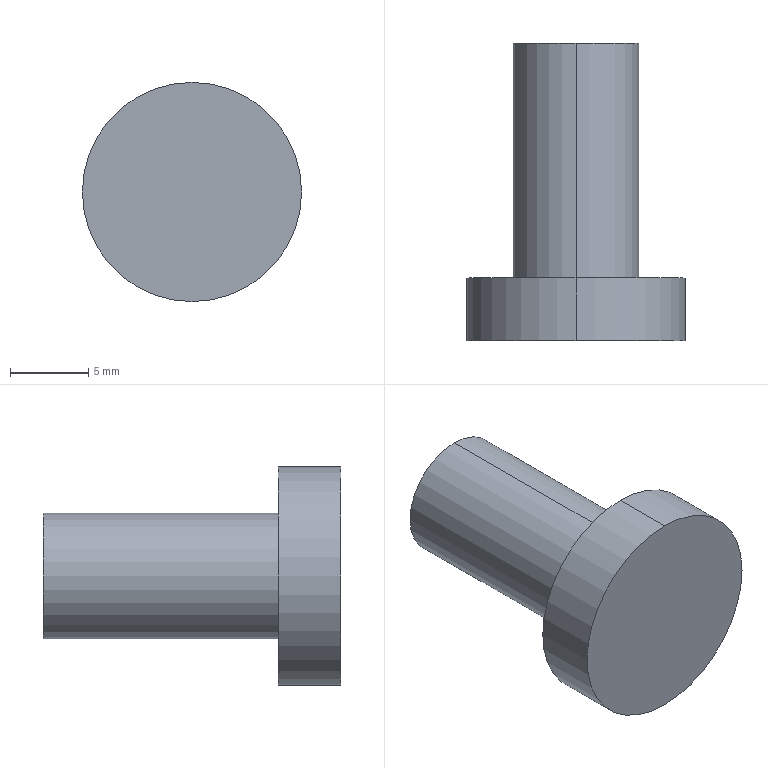Part | STEP file | BU-C03b | 1 solid | 7 faces | box 14 x 19 x 14 mm | volume 1370 mm3 | cylinder 4 | plane 3 | commonest cylinder face diameters 8 x2 14 x2
STEP:
#1=CARTESIAN_POINT('',(0.,0.,0.));
#2=DIRECTION('',(0.,0.,1.));
#3=DIRECTION('',(1.,0.,0.));
#4=AXIS2_PLACEMENT_3D('',#1,#2,#3);
#5=CARTESIAN_POINT('',(0.,4.,4.));
#6=VERTEX_POINT('',#5);
#7=CARTESIAN_POINT('',(0.,4.,-4.));
#8=VERTEX_POINT('',#7);
#9=CARTESIAN_POINT('',(0.,4.,0.));
#10=DIRECTION('',(0.,1.,0.));
#11=DIRECTION('',(0.,0.,1.));
#12=AXIS2_PLACEMENT_3D('',#9,#10,#11);
#13=CIRCLE('',#12,4.);
#14=CARTESIAN_POINT('',(0.,28.998,0.));
#15=DIRECTION('',(0.,1.,0.));
#16=DIRECTION('',(0.,0.,1.));
#17=AXIS2_PLACEMENT_3D('',#14,#15,#16);
#18=CYLINDRICAL_SURFACE('',#17,4.);
#19=CARTESIAN_POINT('',(0.,-24.998));
#20=DIRECTION('',(1.,0.));
#21=VECTOR('',#20,1.);
#22=LINE('',#19,#21);
#23=(GEOMETRIC_REPRESENTATION_CONTEXT(2)PARAMETRIC_REPRESENTATION_CONTEXT()REPRESENTATION_CONTEXT('',''));
#24=DEFINITIONAL_REPRESENTATION('',(#22),#23);
#25=PCURVE('',#18,#24);
#26=CARTESIAN_POINT('',(-4.,4.,0.));
#27=DIRECTION('',(0.,1.,0.));
#28=DIRECTION('',(0.,0.,1.));
#29=AXIS2_PLACEMENT_3D('',#26,#27,#28);
#30=PLANE('',#29);
#31=CARTESIAN_POINT('',(0.,4.));
#32=DIRECTION('',(1.,0.));
#33=AXIS2_PLACEMENT_2D('',#31,#32);
#34=CIRCLE('',#33,4.);
#35=(GEOMETRIC_REPRESENTATION_CONTEXT(2)PARAMETRIC_REPRESENTATION_CONTEXT()REPRESENTATION_CONTEXT('',''));
#36=DEFINITIONAL_REPRESENTATION('',(#34),#35);
#37=PCURVE('',#30,#36);
#38=SURFACE_CURVE('',#13,(#25,#37),.PCURVE_S1.);
#39=EDGE_CURVE('',#6,#8,#38,.T.);
#40=ORIENTED_EDGE('',*,*,#39,.T.);
#41=CARTESIAN_POINT('',(0.,19.,-4.));
#42=VERTEX_POINT('',#41);
#43=CARTESIAN_POINT('',(0.,28.998,-4.));
#44=DIRECTION('',(0.,1.,0.));
#45=VECTOR('',#44,1.);
#46=LINE('',#43,#45);
#47=CARTESIAN_POINT('',(3.142,0.));
#48=DIRECTION('',(0.,1.));
#49=VECTOR('',#48,1.);
#50=LINE('',#47,#49);
#51=(GEOMETRIC_REPRESENTATION_CONTEXT(2)PARAMETRIC_REPRESENTATION_CONTEXT()REPRESENTATION_CONTEXT('',''));
#52=DEFINITIONAL_REPRESENTATION('',(#50),#51);
#53=PCURVE('',#18,#52);
#54=CARTESIAN_POINT('',(0.,28.998,0.));
#55=DIRECTION('',(0.,1.,0.));
#56=DIRECTION('',(0.,0.,1.));
#57=AXIS2_PLACEMENT_3D('',#54,#55,#56);
#58=CYLINDRICAL_SURFACE('',#57,4.);
#59=CARTESIAN_POINT('',(3.142,0.));
#60=DIRECTION('',(0.,1.));
#61=VECTOR('',#60,1.);
#62=LINE('',#59,#61);
#63=(GEOMETRIC_REPRESENTATION_CONTEXT(2)PARAMETRIC_REPRESENTATION_CONTEXT()REPRESENTATION_CONTEXT('',''));
#64=DEFINITIONAL_REPRESENTATION('',(#62),#63);
#65=PCURVE('',#58,#64);
#66=SURFACE_CURVE('',#46,(#53,#65),.PCURVE_S1.);
#67=EDGE_CURVE('',#8,#42,#66,.T.);
#68=ORIENTED_EDGE('',*,*,#67,.T.);
#69=CARTESIAN_POINT('',(0.,19.,4.));
#70=VERTEX_POINT('',#69);
#71=CARTESIAN_POINT('',(0.,19.,0.));
#72=DIRECTION('',(0.,1.,0.));
#73=DIRECTION('',(0.,0.,1.));
#74=AXIS2_PLACEMENT_3D('',#71,#72,#73);
#75=CIRCLE('',#74,4.);
#76=CARTESIAN_POINT('',(0.,-9.998));
#77=DIRECTION('',(1.,0.));
#78=VECTOR('',#77,1.);
#79=LINE('',#76,#78);
#80=(GEOMETRIC_REPRESENTATION_CONTEXT(2)PARAMETRIC_REPRESENTATION_CONTEXT()REPRESENTATION_CONTEXT('',''));
#81=DEFINITIONAL_REPRESENTATION('',(#79),#80);
#82=PCURVE('',#18,#81);
#83=CARTESIAN_POINT('',(-4.,19.,0.));
#84=DIRECTION('',(0.,1.,0.));
#85=DIRECTION('',(0.,0.,1.));
#86=AXIS2_PLACEMENT_3D('',#83,#84,#85);
#87=PLANE('',#86);
#88=CARTESIAN_POINT('',(0.,4.));
#89=DIRECTION('',(1.,0.));
#90=AXIS2_PLACEMENT_2D('',#88,#89);
#91=CIRCLE('',#90,4.);
#92=(GEOMETRIC_REPRESENTATION_CONTEXT(2)PARAMETRIC_REPRESENTATION_CONTEXT()REPRESENTATION_CONTEXT('',''));
#93=DEFINITIONAL_REPRESENTATION('',(#91),#92);
#94=PCURVE('',#87,#93);
#95=SURFACE_CURVE('',#75,(#82,#94),.PCURVE_S1.);
#96=EDGE_CURVE('',#70,#42,#95,.T.);
#97=ORIENTED_EDGE('',*,*,#96,.F.);
#98=CARTESIAN_POINT('',(0.,28.998,4.));
#99=DIRECTION('',(0.,1.,0.));
#100=VECTOR('',#99,1.);
#101=LINE('',#98,#100);
#102=CARTESIAN_POINT('',(0.,0.));
#103=DIRECTION('',(0.,1.));
#104=VECTOR('',#103,1.);
#105=LINE('',#102,#104);
#106=(GEOMETRIC_REPRESENTATION_CONTEXT(2)PARAMETRIC_REPRESENTATION_CONTEXT()REPRESENTATION_CONTEXT('',''));
#107=DEFINITIONAL_REPRESENTATION('',(#105),#106);
#108=PCURVE('',#18,#107);
#109=CARTESIAN_POINT('',(6.283,0.));
#110=DIRECTION('',(0.,1.));
#111=VECTOR('',#110,1.);
#112=LINE('',#109,#111);
#113=(GEOMETRIC_REPRESENTATION_CONTEXT(2)PARAMETRIC_REPRESENTATION_CONTEXT()REPRESENTATION_CONTEXT('',''));
#114=DEFINITIONAL_REPRESENTATION('',(#112),#113);
#115=PCURVE('',#58,#114);
#116=SURFACE_CURVE('',#101,(#108,#115),.PCURVE_S1.);
#117=EDGE_CURVE('',#6,#70,#116,.T.);
#118=ORIENTED_EDGE('',*,*,#117,.F.);
#119=EDGE_LOOP('',(#40,#68,#97,#118));
#120=FACE_BOUND('',#119,.T.);
#121=ADVANCED_FACE('',(#120),#18,.T.);
#122=CARTESIAN_POINT('',(0.,0.,7.));
#123=VERTEX_POINT('',#122);
#124=CARTESIAN_POINT('',(0.,0.,-7.));
#125=VERTEX_POINT('',#124);
#126=CARTESIAN_POINT('',(0.,0.,0.));
#127=DIRECTION('',(0.,1.,0.));
#128=DIRECTION('',(0.,0.,1.));
#129=AXIS2_PLACEMENT_3D('',#126,#127,#128);
#130=CIRCLE('',#129,7.);
#131=CARTESIAN_POINT('',(0.,28.998,0.));
#132=DIRECTION('',(0.,1.,0.));
#133=DIRECTION('',(0.,0.,1.));
#134=AXIS2_PLACEMENT_3D('',#131,#132,#133);
#135=CYLINDRICAL_SURFACE('',#134,7.);
#136=CARTESIAN_POINT('',(0.,-28.998));
#137=DIRECTION('',(1.,0.));
#138=VECTOR('',#137,1.);
#139=LINE('',#136,#138);
#140=(GEOMETRIC_REPRESENTATION_CONTEXT(2)PARAMETRIC_REPRESENTATION_CONTEXT()REPRESENTATION_CONTEXT('',''));
#141=DEFINITIONAL_REPRESENTATION('',(#139),#140);
#142=PCURVE('',#135,#141);
#143=CARTESIAN_POINT('',(-7.,0.,0.));
#144=DIRECTION('',(0.,-1.,0.));
#145=DIRECTION('',(0.,0.,-1.));
#146=AXIS2_PLACEMENT_3D('',#143,#144,#145);
#147=PLANE('',#146);
#148=CARTESIAN_POINT('',(-7.,7.));
#149=CARTESIAN_POINT('',(-7.,19.124));
#150=CARTESIAN_POINT('',(3.5,13.062));
#151=CARTESIAN_POINT('',(14.,7.));
#152=CARTESIAN_POINT('',(3.5,0.9378));
#153=CARTESIAN_POINT('',(-7.,-5.124));
#154=CARTESIAN_POINT('',(-7.,7.));
#155=(BOUNDED_CURVE()B_SPLINE_CURVE(2,(#148,#149,#150,#151,#152,#153,#154),.UNSPECIFIED.,.T.,.F.)B_SPLINE_CURVE_WITH_KNOTS((1,2,2,2,2,1),(-2.094,0.,2.094,4.189,6.283,8.378),.UNSPECIFIED.)CURVE()GEOMETRIC_REPRESENTATION_ITEM()RATIONAL_B_SPLINE_CURVE((1.,0.5,1.,0.5,1.,0.5,1.))REPRESENTATION_ITEM(''));
#156=(GEOMETRIC_REPRESENTATION_CONTEXT(2)PARAMETRIC_REPRESENTATION_CONTEXT()REPRESENTATION_CONTEXT('',''));
#157=DEFINITIONAL_REPRESENTATION('',(#155),#156);
#158=PCURVE('',#147,#157);
#159=SURFACE_CURVE('',#130,(#142,#158),.PCURVE_S1.);
#160=EDGE_CURVE('',#123,#125,#159,.T.);
#161=ORIENTED_EDGE('',*,*,#160,.T.);
#162=CARTESIAN_POINT('',(0.,4.,-7.));
#163=VERTEX_POINT('',#162);
#164=CARTESIAN_POINT('',(0.,28.998,-7.));
#165=DIRECTION('',(0.,1.,0.));
#166=VECTOR('',#165,1.);
#167=LINE('',#164,#166);
#168=CARTESIAN_POINT('',(3.142,0.));
#169=DIRECTION('',(0.,1.));
#170=VECTOR('',#169,1.);
#171=LINE('',#168,#170);
#172=(GEOMETRIC_REPRESENTATION_CONTEXT(2)PARAMETRIC_REPRESENTATION_CONTEXT()REPRESENTATION_CONTEXT('',''));
#173=DEFINITIONAL_REPRESENTATION('',(#171),#172);
#174=PCURVE('',#135,#173);
#175=CARTESIAN_POINT('',(0.,28.998,0.));
#176=DIRECTION('',(0.,1.,0.));
#177=DIRECTION('',(0.,0.,1.));
#178=AXIS2_PLACEMENT_3D('',#175,#176,#177);
#179=CYLINDRICAL_SURFACE('',#178,7.);
#180=CARTESIAN_POINT('',(3.142,0.));
#181=DIRECTION('',(0.,1.));
#182=VECTOR('',#181,1.);
#183=LINE('',#180,#182);
#184=(GEOMETRIC_REPRESENTATION_CONTEXT(2)PARAMETRIC_REPRESENTATION_CONTEXT()REPRESENTATION_CONTEXT('',''));
#185=DEFINITIONAL_REPRESENTATION('',(#183),#184);
#186=PCURVE('',#179,#185);
#187=SURFACE_CURVE('',#167,(#174,#186),.PCURVE_S1.);
#188=EDGE_CURVE('',#125,#163,#187,.T.);
#189=ORIENTED_EDGE('',*,*,#188,.T.);
#190=CARTESIAN_POINT('',(0.,4.,7.));
#191=VERTEX_POINT('',#190);
#192=CARTESIAN_POINT('',(0.,4.,0.));
#193=DIRECTION('',(0.,1.,0.));
#194=DIRECTION('',(0.,0.,1.));
#195=AXIS2_PLACEMENT_3D('',#192,#193,#194);
#196=CIRCLE('',#195,7.);
#197=CARTESIAN_POINT('',(0.,-24.998));
#198=DIRECTION('',(1.,0.));
#199=VECTOR('',#198,1.);
#200=LINE('',#197,#199);
#201=(GEOMETRIC_REPRESENTATION_CONTEXT(2)PARAMETRIC_REPRESENTATION_CONTEXT()REPRESENTATION_CONTEXT('',''));
#202=DEFINITIONAL_REPRESENTATION('',(#200),#201);
#203=PCURVE('',#135,#202);
#204=CARTESIAN_POINT('',(0.,4.));
#205=DIRECTION('',(1.,0.));
#206=AXIS2_PLACEMENT_2D('',#204,#205);
#207=CIRCLE('',#206,7.);
#208=(GEOMETRIC_REPRESENTATION_CONTEXT(2)PARAMETRIC_REPRESENTATION_CONTEXT()REPRESENTATION_CONTEXT('',''));
#209=DEFINITIONAL_REPRESENTATION('',(#207),#208);
#210=PCURVE('',#30,#209);
#211=SURFACE_CURVE('',#196,(#203,#210),.PCURVE_S1.);
#212=EDGE_CURVE('',#191,#163,#211,.T.);
#213=ORIENTED_EDGE('',*,*,#212,.F.);
#214=CARTESIAN_POINT('',(0.,28.998,7.));
#215=DIRECTION('',(0.,1.,0.));
#216=VECTOR('',#215,1.);
#217=LINE('',#214,#216);
#218=CARTESIAN_POINT('',(0.,0.));
#219=DIRECTION('',(0.,1.));
#220=VECTOR('',#219,1.);
#221=LINE('',#218,#220);
#222=(GEOMETRIC_REPRESENTATION_CONTEXT(2)PARAMETRIC_REPRESENTATION_CONTEXT()REPRESENTATION_CONTEXT('',''));
#223=DEFINITIONAL_REPRESENTATION('',(#221),#222);
#224=PCURVE('',#135,#223);
#225=CARTESIAN_POINT('',(6.283,0.));
#226=DIRECTION('',(0.,1.));
#227=VECTOR('',#226,1.);
#228=LINE('',#225,#227);
#229=(GEOMETRIC_REPRESENTATION_CONTEXT(2)PARAMETRIC_REPRESENTATION_CONTEXT()REPRESENTATION_CONTEXT('',''));
#230=DEFINITIONAL_REPRESENTATION('',(#228),#229);
#231=PCURVE('',#179,#230);
#232=SURFACE_CURVE('',#217,(#224,#231),.PCURVE_S1.);
#233=EDGE_CURVE('',#123,#191,#232,.T.);
#234=ORIENTED_EDGE('',*,*,#233,.F.);
#235=EDGE_LOOP('',(#161,#189,#213,#234));
#236=FACE_BOUND('',#235,.T.);
#237=ADVANCED_FACE('',(#236),#135,.T.);
#238=ORIENTED_EDGE('',*,*,#96,.T.);
#239=CARTESIAN_POINT('',(0.,19.,0.));
#240=DIRECTION('',(0.,1.,0.));
#241=DIRECTION('',(0.,0.,1.));
#242=AXIS2_PLACEMENT_3D('',#239,#240,#241);
#243=CIRCLE('',#242,4.);
#244=CARTESIAN_POINT('',(0.,4.));
#245=DIRECTION('',(1.,0.));
#246=AXIS2_PLACEMENT_2D('',#244,#245);
#247=CIRCLE('',#246,4.);
#248=(GEOMETRIC_REPRESENTATION_CONTEXT(2)PARAMETRIC_REPRESENTATION_CONTEXT()REPRESENTATION_CONTEXT('',''));
#249=DEFINITIONAL_REPRESENTATION('',(#247),#248);
#250=PCURVE('',#87,#249);
#251=CARTESIAN_POINT('',(0.,-9.998));
#252=DIRECTION('',(1.,0.));
#253=VECTOR('',#252,1.);
#254=LINE('',#251,#253);
#255=(GEOMETRIC_REPRESENTATION_CONTEXT(2)PARAMETRIC_REPRESENTATION_CONTEXT()REPRESENTATION_CONTEXT('',''));
#256=DEFINITIONAL_REPRESENTATION('',(#254),#255);
#257=PCURVE('',#58,#256);
#258=SURFACE_CURVE('',#243,(#250,#257),.PCURVE_S1.);
#259=EDGE_CURVE('',#42,#70,#258,.T.);
#260=ORIENTED_EDGE('',*,*,#259,.T.);
#261=EDGE_LOOP('',(#238,#260));
#262=FACE_BOUND('',#261,.T.);
#263=ADVANCED_FACE('',(#262),#87,.T.);
#264=ORIENTED_EDGE('',*,*,#160,.F.);
#265=CARTESIAN_POINT('',(0.,0.,0.));
#266=DIRECTION('',(0.,1.,0.));
#267=DIRECTION('',(0.,0.,1.));
#268=AXIS2_PLACEMENT_3D('',#265,#266,#267);
#269=CIRCLE('',#268,7.);
#270=CARTESIAN_POINT('',(-7.,7.));
#271=CARTESIAN_POINT('',(-7.,19.124));
#272=CARTESIAN_POINT('',(3.5,13.062));
#273=CARTESIAN_POINT('',(14.,7.));
#274=CARTESIAN_POINT('',(3.5,0.9378));
#275=CARTESIAN_POINT('',(-7.,-5.124));
#276=CARTESIAN_POINT('',(-7.,7.));
#277=(BOUNDED_CURVE()B_SPLINE_CURVE(2,(#270,#271,#272,#273,#274,#275,#276),.UNSPECIFIED.,.T.,.F.)B_SPLINE_CURVE_WITH_KNOTS((1,2,2,2,2,1),(-2.094,0.,2.094,4.189,6.283,8.378),.UNSPECIFIED.)CURVE()GEOMETRIC_REPRESENTATION_ITEM()RATIONAL_B_SPLINE_CURVE((1.,0.5,1.,0.5,1.,0.5,1.))REPRESENTATION_ITEM(''));
#278=(GEOMETRIC_REPRESENTATION_CONTEXT(2)PARAMETRIC_REPRESENTATION_CONTEXT()REPRESENTATION_CONTEXT('',''));
#279=DEFINITIONAL_REPRESENTATION('',(#277),#278);
#280=PCURVE('',#147,#279);
#281=CARTESIAN_POINT('',(0.,-28.998));
#282=DIRECTION('',(1.,0.));
#283=VECTOR('',#282,1.);
#284=LINE('',#281,#283);
#285=(GEOMETRIC_REPRESENTATION_CONTEXT(2)PARAMETRIC_REPRESENTATION_CONTEXT()REPRESENTATION_CONTEXT('',''));
#286=DEFINITIONAL_REPRESENTATION('',(#284),#285);
#287=PCURVE('',#179,#286);
#288=SURFACE_CURVE('',#269,(#280,#287),.PCURVE_S1.);
#289=EDGE_CURVE('',#125,#123,#288,.T.);
#290=ORIENTED_EDGE('',*,*,#289,.F.);
#291=EDGE_LOOP('',(#264,#290));
#292=FACE_BOUND('',#291,.T.);
#293=ADVANCED_FACE('',(#292),#147,.T.);
#294=ORIENTED_EDGE('',*,*,#188,.F.);
#295=ORIENTED_EDGE('',*,*,#289,.T.);
#296=ORIENTED_EDGE('',*,*,#233,.T.);
#297=CARTESIAN_POINT('',(0.,4.,0.));
#298=DIRECTION('',(0.,1.,0.));
#299=DIRECTION('',(0.,0.,1.));
#300=AXIS2_PLACEMENT_3D('',#297,#298,#299);
#301=CIRCLE('',#300,7.);
#302=CARTESIAN_POINT('',(0.,-24.998));
#303=DIRECTION('',(1.,0.));
#304=VECTOR('',#303,1.);
#305=LINE('',#302,#304);
#306=(GEOMETRIC_REPRESENTATION_CONTEXT(2)PARAMETRIC_REPRESENTATION_CONTEXT()REPRESENTATION_CONTEXT('',''));
#307=DEFINITIONAL_REPRESENTATION('',(#305),#306);
#308=PCURVE('',#179,#307);
#309=CARTESIAN_POINT('',(0.,4.));
#310=DIRECTION('',(1.,0.));
#311=AXIS2_PLACEMENT_2D('',#309,#310);
#312=CIRCLE('',#311,7.);
#313=(GEOMETRIC_REPRESENTATION_CONTEXT(2)PARAMETRIC_REPRESENTATION_CONTEXT()REPRESENTATION_CONTEXT('',''));
#314=DEFINITIONAL_REPRESENTATION('',(#312),#313);
#315=PCURVE('',#30,#314);
#316=SURFACE_CURVE('',#301,(#308,#315),.PCURVE_S1.);
#317=EDGE_CURVE('',#163,#191,#316,.T.);
#318=ORIENTED_EDGE('',*,*,#317,.F.);
#319=EDGE_LOOP('',(#294,#295,#296,#318));
#320=FACE_BOUND('',#319,.T.);
#321=ADVANCED_FACE('',(#320),#179,.T.);
#322=ORIENTED_EDGE('',*,*,#212,.T.);
#323=ORIENTED_EDGE('',*,*,#317,.T.);
#324=EDGE_LOOP('',(#322,#323));
#325=FACE_BOUND('',#324,.T.);
#326=ORIENTED_EDGE('',*,*,#39,.F.);
#327=CARTESIAN_POINT('',(0.,4.,0.));
#328=DIRECTION('',(0.,1.,0.));
#329=DIRECTION('',(0.,0.,1.));
#330=AXIS2_PLACEMENT_3D('',#327,#328,#329);
#331=CIRCLE('',#330,4.);
#332=CARTESIAN_POINT('',(0.,4.));
#333=DIRECTION('',(1.,0.));
#334=AXIS2_PLACEMENT_2D('',#332,#333);
#335=CIRCLE('',#334,4.);
#336=(GEOMETRIC_REPRESENTATION_CONTEXT(2)PARAMETRIC_REPRESENTATION_CONTEXT()REPRESENTATION_CONTEXT('',''));
#337=DEFINITIONAL_REPRESENTATION('',(#335),#336);
#338=PCURVE('',#30,#337);
#339=CARTESIAN_POINT('',(0.,-24.998));
#340=DIRECTION('',(1.,0.));
#341=VECTOR('',#340,1.);
#342=LINE('',#339,#341);
#343=(GEOMETRIC_REPRESENTATION_CONTEXT(2)PARAMETRIC_REPRESENTATION_CONTEXT()REPRESENTATION_CONTEXT('',''));
#344=DEFINITIONAL_REPRESENTATION('',(#342),#343);
#345=PCURVE('',#58,#344);
#346=SURFACE_CURVE('',#331,(#338,#345),.PCURVE_S1.);
#347=EDGE_CURVE('',#8,#6,#346,.T.);
#348=ORIENTED_EDGE('',*,*,#347,.F.);
#349=EDGE_LOOP('',(#326,#348));
#350=FACE_BOUND('',#349,.T.);
#351=ADVANCED_FACE('',(#325,#350),#30,.T.);
#352=ORIENTED_EDGE('',*,*,#67,.F.);
#353=ORIENTED_EDGE('',*,*,#347,.T.);
#354=ORIENTED_EDGE('',*,*,#117,.T.);
#355=ORIENTED_EDGE('',*,*,#259,.F.);
#356=EDGE_LOOP('',(#352,#353,#354,#355));
#357=FACE_BOUND('',#356,.T.);
#358=ADVANCED_FACE('',(#357),#58,.T.);
#359=CLOSED_SHELL('',(#121,#237,#263,#293,#321,#351,#358));
#360=MANIFOLD_SOLID_BREP('',#359);
#361=(LENGTH_UNIT()NAMED_UNIT(*)SI_UNIT(.MILLI.,.METRE.));
#362=UNCERTAINTY_MEASURE_WITH_UNIT(LENGTH_MEASURE(0.0000001),#361,'','');
#363=(NAMED_UNIT(*)PLANE_ANGLE_UNIT()SI_UNIT($,.RADIAN.));
#364=(NAMED_UNIT(*)SI_UNIT($,.STERADIAN.)SOLID_ANGLE_UNIT());
#365=(GEOMETRIC_REPRESENTATION_CONTEXT(3)GLOBAL_UNCERTAINTY_ASSIGNED_CONTEXT((#362))GLOBAL_UNIT_ASSIGNED_CONTEXT((#361,#363,#364))REPRESENTATION_CONTEXT('',''));
#366=ADVANCED_BREP_SHAPE_REPRESENTATION('',(#4,#360),#365);